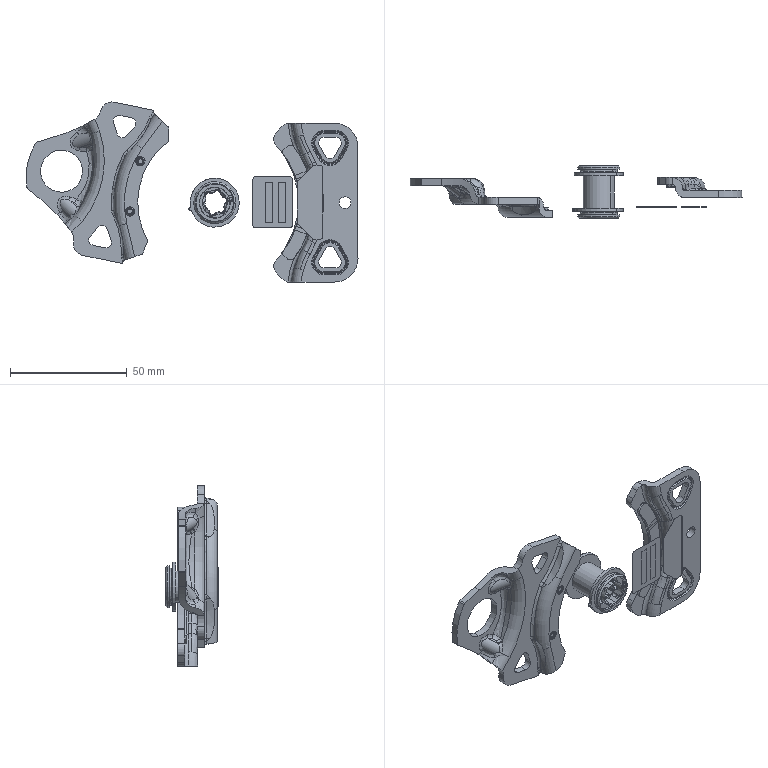Part | NX | features BREP 6 | 7 solids | 1006 faces | box 142.204 x 22.65 x 77.146 mm | volume 17017 mm3 | cylinder 403 | plane 259 | spline 158 | torus 104 | cone 66 | sphere 16 | commonest cylinder face diameters 0.3 x80 0.6 x78 1 x25 4 x18 3 x16 1.6 x15